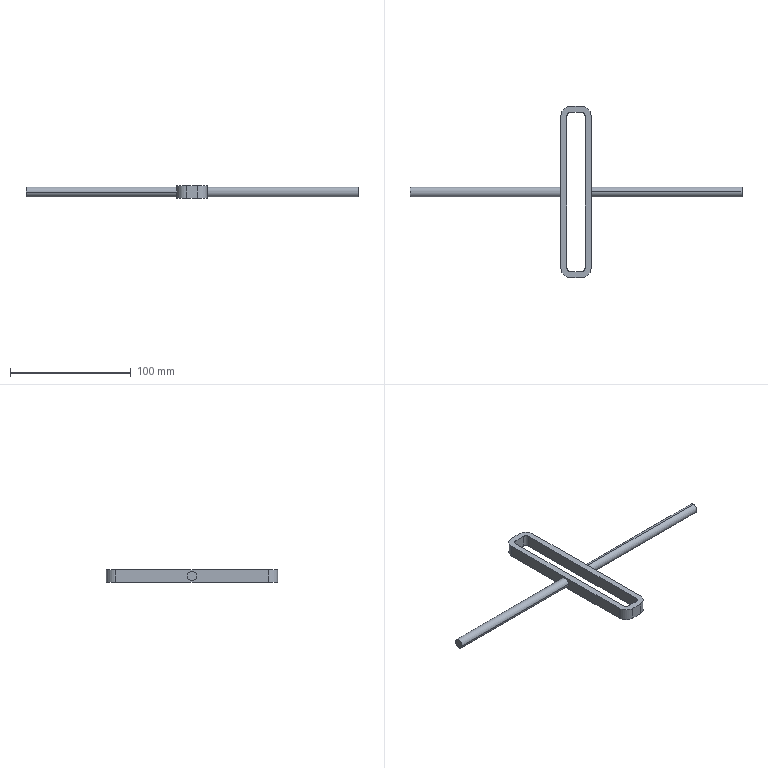Part | SolidWorks | features ICE 2, Extrusion 1 | 1 solid | 24 faces | box 275 x 142 x 10 mm | volume 27794 mm3 | cylinder 12 | plane 12 | commonest cylinder face diameters 6 x4 8 x4 16 x4
STEP:
#1=CARTESIAN_POINT('',(-137.5,-4.,5.));
#2=VERTEX_POINT('',#1);
#3=CARTESIAN_POINT('',(-137.5,4.,5.));
#4=VERTEX_POINT('',#3);
#5=CARTESIAN_POINT('',(-137.5,0.,5.));
#6=DIRECTION('',(-1.,0.,0.));
#7=DIRECTION('',(0.,-1.,0.));
#8=AXIS2_PLACEMENT_3D('',#5,#6,#7);
#9=CIRCLE('',#8,4.);
#10=EDGE_CURVE('',#2,#4,#9,.T.);
#11=ORIENTED_EDGE('',*,*,#10,.F.);
#12=CARTESIAN_POINT('',(-12.5,-4.,5.));
#13=VERTEX_POINT('',#12);
#14=CARTESIAN_POINT('',(-137.5,-4.,5.));
#15=DIRECTION('',(1.,0.,0.));
#16=VECTOR('',#15,1000.);
#17=LINE('',#14,#16);
#18=EDGE_CURVE('',#2,#13,#17,.T.);
#19=ORIENTED_EDGE('',*,*,#18,.T.);
#20=CARTESIAN_POINT('',(-12.5,4.,5.));
#21=VERTEX_POINT('',#20);
#22=CARTESIAN_POINT('',(-12.5,0.,5.));
#23=DIRECTION('',(-1.,0.,0.));
#24=DIRECTION('',(0.,1.,0.));
#25=AXIS2_PLACEMENT_3D('',#22,#23,#24);
#26=CIRCLE('',#25,4.);
#27=EDGE_CURVE('',#13,#21,#26,.T.);
#28=ORIENTED_EDGE('',*,*,#27,.T.);
#29=CARTESIAN_POINT('',(-137.5,4.,5.));
#30=DIRECTION('',(1.,0.,0.));
#31=VECTOR('',#30,1000.);
#32=LINE('',#29,#31);
#33=EDGE_CURVE('',#4,#21,#32,.T.);
#34=ORIENTED_EDGE('',*,*,#33,.F.);
#35=EDGE_LOOP('',(#11,#19,#28,#34));
#36=FACE_OUTER_BOUND('',#35,.T.);
#37=CARTESIAN_POINT('',(-137.5,0.,5.));
#38=DIRECTION('',(1.,0.,0.));
#39=DIRECTION('',(0.,1.,0.));
#40=AXIS2_PLACEMENT_3D('',#37,#38,#39);
#41=CYLINDRICAL_SURFACE('',#40,4.);
#42=ADVANCED_FACE('',(#36),#41,.T.);
#43=CARTESIAN_POINT('',(137.5,0.,1.));
#44=VERTEX_POINT('',#43);
#45=CARTESIAN_POINT('',(137.5,0.,9.));
#46=VERTEX_POINT('',#45);
#47=CARTESIAN_POINT('',(137.5,0.,5.));
#48=DIRECTION('',(1.,0.,0.));
#49=DIRECTION('',(0.,0.,-1.));
#50=AXIS2_PLACEMENT_3D('',#47,#48,#49);
#51=CIRCLE('',#50,4.);
#52=EDGE_CURVE('',#44,#46,#51,.T.);
#53=ORIENTED_EDGE('',*,*,#52,.F.);
#54=CARTESIAN_POINT('',(12.5,0.,1.));
#55=VERTEX_POINT('',#54);
#56=CARTESIAN_POINT('',(137.5,0.,1.));
#57=DIRECTION('',(-1.,0.,0.));
#58=VECTOR('',#57,1000.);
#59=LINE('',#56,#58);
#60=EDGE_CURVE('',#44,#55,#59,.T.);
#61=ORIENTED_EDGE('',*,*,#60,.T.);
#62=CARTESIAN_POINT('',(12.5,0.,9.));
#63=VERTEX_POINT('',#62);
#64=CARTESIAN_POINT('',(12.5,0.,5.));
#65=DIRECTION('',(1.,0.,0.));
#66=DIRECTION('',(0.,-1.,0.));
#67=AXIS2_PLACEMENT_3D('',#64,#65,#66);
#68=CIRCLE('',#67,4.);
#69=EDGE_CURVE('',#55,#63,#68,.T.);
#70=ORIENTED_EDGE('',*,*,#69,.T.);
#71=CARTESIAN_POINT('',(137.5,0.,9.));
#72=DIRECTION('',(-1.,0.,0.));
#73=VECTOR('',#72,1000.);
#74=LINE('',#71,#73);
#75=EDGE_CURVE('',#46,#63,#74,.T.);
#76=ORIENTED_EDGE('',*,*,#75,.F.);
#77=EDGE_LOOP('',(#53,#61,#70,#76));
#78=FACE_OUTER_BOUND('',#77,.T.);
#79=CARTESIAN_POINT('',(137.5,0.,5.));
#80=DIRECTION('',(-1.,0.,0.));
#81=DIRECTION('',(0.,0.,1.));
#82=AXIS2_PLACEMENT_3D('',#79,#80,#81);
#83=CYLINDRICAL_SURFACE('',#82,4.);
#84=ADVANCED_FACE('',(#78),#83,.T.);
#85=CARTESIAN_POINT('',(-4.5,71.,10.));
#86=VERTEX_POINT('',#85);
#87=CARTESIAN_POINT('',(-12.5,63.,10.));
#88=VERTEX_POINT('',#87);
#89=CARTESIAN_POINT('',(-4.5,63.,10.));
#90=DIRECTION('',(0.,0.,1.));
#91=DIRECTION('',(1.,0.,0.));
#92=AXIS2_PLACEMENT_3D('',#89,#90,#91);
#93=CIRCLE('',#92,8.);
#94=EDGE_CURVE('',#86,#88,#93,.T.);
#95=ORIENTED_EDGE('',*,*,#94,.T.);
#96=CARTESIAN_POINT('',(-12.5,-63.,10.));
#97=VERTEX_POINT('',#96);
#98=CARTESIAN_POINT('',(-12.5,63.,10.));
#99=DIRECTION('',(0.,-1.,0.));
#100=VECTOR('',#99,1000.);
#101=LINE('',#98,#100);
#102=EDGE_CURVE('',#88,#97,#101,.T.);
#103=ORIENTED_EDGE('',*,*,#102,.T.);
#104=CARTESIAN_POINT('',(-4.5,-71.,10.));
#105=VERTEX_POINT('',#104);
#106=CARTESIAN_POINT('',(-4.5,-63.,10.));
#107=DIRECTION('',(0.,0.,1.));
#108=DIRECTION('',(1.,0.,0.));
#109=AXIS2_PLACEMENT_3D('',#106,#107,#108);
#110=CIRCLE('',#109,8.);
#111=EDGE_CURVE('',#97,#105,#110,.T.);
#112=ORIENTED_EDGE('',*,*,#111,.T.);
#113=CARTESIAN_POINT('',(4.5,-71.,10.));
#114=VERTEX_POINT('',#113);
#115=CARTESIAN_POINT('',(-4.5,-71.,10.));
#116=DIRECTION('',(1.,0.,0.));
#117=VECTOR('',#116,1000.);
#118=LINE('',#115,#117);
#119=EDGE_CURVE('',#105,#114,#118,.T.);
#120=ORIENTED_EDGE('',*,*,#119,.T.);
#121=CARTESIAN_POINT('',(12.5,-63.,10.));
#122=VERTEX_POINT('',#121);
#123=CARTESIAN_POINT('',(4.5,-63.,10.));
#124=DIRECTION('',(0.,0.,1.));
#125=DIRECTION('',(1.,0.,0.));
#126=AXIS2_PLACEMENT_3D('',#123,#124,#125);
#127=CIRCLE('',#126,8.);
#128=EDGE_CURVE('',#114,#122,#127,.T.);
#129=ORIENTED_EDGE('',*,*,#128,.T.);
#130=CARTESIAN_POINT('',(12.5,63.,10.));
#131=VERTEX_POINT('',#130);
#132=CARTESIAN_POINT('',(12.5,63.,10.));
#133=DIRECTION('',(0.,1.,0.));
#134=VECTOR('',#133,1000.);
#135=LINE('',#132,#134);
#136=EDGE_CURVE('',#122,#131,#135,.T.);
#137=ORIENTED_EDGE('',*,*,#136,.T.);
#138=CARTESIAN_POINT('',(4.5,71.,10.));
#139=VERTEX_POINT('',#138);
#140=CARTESIAN_POINT('',(4.5,63.,10.));
#141=DIRECTION('',(0.,0.,1.));
#142=DIRECTION('',(-1.,0.,0.));
#143=AXIS2_PLACEMENT_3D('',#140,#141,#142);
#144=CIRCLE('',#143,8.);
#145=EDGE_CURVE('',#131,#139,#144,.T.);
#146=ORIENTED_EDGE('',*,*,#145,.T.);
#147=CARTESIAN_POINT('',(-4.5,71.,10.));
#148=DIRECTION('',(-1.,0.,0.));
#149=VECTOR('',#148,1000.);
#150=LINE('',#147,#149);
#151=EDGE_CURVE('',#139,#86,#150,.T.);
#152=ORIENTED_EDGE('',*,*,#151,.T.);
#153=EDGE_LOOP('',(#95,#103,#112,#120,#129,#137,#146,#152));
#154=FACE_OUTER_BOUND('',#153,.T.);
#155=CARTESIAN_POINT('',(-4.5,-66.,10.));
#156=VERTEX_POINT('',#155);
#157=CARTESIAN_POINT('',(4.5,-66.,10.));
#158=VERTEX_POINT('',#157);
#159=CARTESIAN_POINT('',(-4.5,-66.,10.));
#160=DIRECTION('',(1.,0.,0.));
#161=VECTOR('',#160,1000.);
#162=LINE('',#159,#161);
#163=EDGE_CURVE('',#156,#158,#162,.T.);
#164=ORIENTED_EDGE('',*,*,#163,.F.);
#165=CARTESIAN_POINT('',(-7.5,-63.,10.));
#166=VERTEX_POINT('',#165);
#167=CARTESIAN_POINT('',(-4.5,-63.,10.));
#168=DIRECTION('',(0.,0.,1.));
#169=DIRECTION('',(1.,0.,0.));
#170=AXIS2_PLACEMENT_3D('',#167,#168,#169);
#171=CIRCLE('',#170,3.);
#172=EDGE_CURVE('',#166,#156,#171,.T.);
#173=ORIENTED_EDGE('',*,*,#172,.F.);
#174=CARTESIAN_POINT('',(-7.5,63.,10.));
#175=VERTEX_POINT('',#174);
#176=CARTESIAN_POINT('',(-7.5,63.,10.));
#177=DIRECTION('',(0.,-1.,0.));
#178=VECTOR('',#177,1000.);
#179=LINE('',#176,#178);
#180=EDGE_CURVE('',#175,#166,#179,.T.);
#181=ORIENTED_EDGE('',*,*,#180,.F.);
#182=CARTESIAN_POINT('',(-4.5,66.,10.));
#183=VERTEX_POINT('',#182);
#184=CARTESIAN_POINT('',(-4.5,63.,10.));
#185=DIRECTION('',(0.,0.,1.));
#186=DIRECTION('',(1.,0.,0.));
#187=AXIS2_PLACEMENT_3D('',#184,#185,#186);
#188=CIRCLE('',#187,3.);
#189=EDGE_CURVE('',#183,#175,#188,.T.);
#190=ORIENTED_EDGE('',*,*,#189,.F.);
#191=CARTESIAN_POINT('',(4.5,66.,10.));
#192=VERTEX_POINT('',#191);
#193=CARTESIAN_POINT('',(-4.5,66.,10.));
#194=DIRECTION('',(-1.,0.,0.));
#195=VECTOR('',#194,1000.);
#196=LINE('',#193,#195);
#197=EDGE_CURVE('',#192,#183,#196,.T.);
#198=ORIENTED_EDGE('',*,*,#197,.F.);
#199=CARTESIAN_POINT('',(7.5,63.,10.));
#200=VERTEX_POINT('',#199);
#201=CARTESIAN_POINT('',(4.5,63.,10.));
#202=DIRECTION('',(0.,0.,1.));
#203=DIRECTION('',(-1.,0.,0.));
#204=AXIS2_PLACEMENT_3D('',#201,#202,#203);
#205=CIRCLE('',#204,3.);
#206=EDGE_CURVE('',#200,#192,#205,.T.);
#207=ORIENTED_EDGE('',*,*,#206,.F.);
#208=CARTESIAN_POINT('',(7.5,-63.,10.));
#209=VERTEX_POINT('',#208);
#210=CARTESIAN_POINT('',(7.5,63.,10.));
#211=DIRECTION('',(0.,1.,0.));
#212=VECTOR('',#211,1000.);
#213=LINE('',#210,#212);
#214=EDGE_CURVE('',#209,#200,#213,.T.);
#215=ORIENTED_EDGE('',*,*,#214,.F.);
#216=CARTESIAN_POINT('',(4.5,-63.,10.));
#217=DIRECTION('',(0.,0.,1.));
#218=DIRECTION('',(1.,0.,0.));
#219=AXIS2_PLACEMENT_3D('',#216,#217,#218);
#220=CIRCLE('',#219,3.);
#221=EDGE_CURVE('',#158,#209,#220,.T.);
#222=ORIENTED_EDGE('',*,*,#221,.F.);
#223=EDGE_LOOP('',(#164,#173,#181,#190,#198,#207,#215,#222));
#224=FACE_BOUND('',#223,.T.);
#225=CARTESIAN_POINT('',(-4.5,63.,10.));
#226=DIRECTION('',(0.,0.,1.));
#227=DIRECTION('',(1.,0.,0.));
#228=AXIS2_PLACEMENT_3D('',#225,#226,#227);
#229=PLANE('',#228);
#230=ADVANCED_FACE('',(#154,#224),#229,.T.);
#231=CARTESIAN_POINT('',(-4.5,71.,0.));
#232=VERTEX_POINT('',#231);
#233=CARTESIAN_POINT('',(-12.5,63.,0.));
#234=VERTEX_POINT('',#233);
#235=CARTESIAN_POINT('',(-4.5,63.,0.));
#236=DIRECTION('',(0.,0.,1.));
#237=DIRECTION('',(1.,0.,0.));
#238=AXIS2_PLACEMENT_3D('',#235,#236,#237);
#239=CIRCLE('',#238,8.);
#240=EDGE_CURVE('',#232,#234,#239,.T.);
#241=ORIENTED_EDGE('',*,*,#240,.F.);
#242=CARTESIAN_POINT('',(4.5,71.,0.));
#243=VERTEX_POINT('',#242);
#244=CARTESIAN_POINT('',(-4.5,71.,0.));
#245=DIRECTION('',(-1.,0.,0.));
#246=VECTOR('',#245,1000.);
#247=LINE('',#244,#246);
#248=EDGE_CURVE('',#243,#232,#247,.T.);
#249=ORIENTED_EDGE('',*,*,#248,.F.);
#250=CARTESIAN_POINT('',(12.5,63.,0.));
#251=VERTEX_POINT('',#250);
#252=CARTESIAN_POINT('',(4.5,63.,0.));
#253=DIRECTION('',(0.,0.,1.));
#254=DIRECTION('',(-1.,0.,0.));
#255=AXIS2_PLACEMENT_3D('',#252,#253,#254);
#256=CIRCLE('',#255,8.);
#257=EDGE_CURVE('',#251,#243,#256,.T.);
#258=ORIENTED_EDGE('',*,*,#257,.F.);
#259=CARTESIAN_POINT('',(12.5,-63.,0.));
#260=VERTEX_POINT('',#259);
#261=CARTESIAN_POINT('',(12.5,63.,0.));
#262=DIRECTION('',(0.,1.,0.));
#263=VECTOR('',#262,1000.);
#264=LINE('',#261,#263);
#265=EDGE_CURVE('',#260,#251,#264,.T.);
#266=ORIENTED_EDGE('',*,*,#265,.F.);
#267=CARTESIAN_POINT('',(4.5,-71.,0.));
#268=VERTEX_POINT('',#267);
#269=CARTESIAN_POINT('',(4.5,-63.,0.));
#270=DIRECTION('',(0.,0.,1.));
#271=DIRECTION('',(1.,0.,0.));
#272=AXIS2_PLACEMENT_3D('',#269,#270,#271);
#273=CIRCLE('',#272,8.);
#274=EDGE_CURVE('',#268,#260,#273,.T.);
#275=ORIENTED_EDGE('',*,*,#274,.F.);
#276=CARTESIAN_POINT('',(-4.5,-71.,0.));
#277=VERTEX_POINT('',#276);
#278=CARTESIAN_POINT('',(-4.5,-71.,0.));
#279=DIRECTION('',(1.,0.,0.));
#280=VECTOR('',#279,1000.);
#281=LINE('',#278,#280);
#282=EDGE_CURVE('',#277,#268,#281,.T.);
#283=ORIENTED_EDGE('',*,*,#282,.F.);
#284=CARTESIAN_POINT('',(-12.5,-63.,0.));
#285=VERTEX_POINT('',#284);
#286=CARTESIAN_POINT('',(-4.5,-63.,0.));
#287=DIRECTION('',(0.,0.,1.));
#288=DIRECTION('',(1.,0.,0.));
#289=AXIS2_PLACEMENT_3D('',#286,#287,#288);
#290=CIRCLE('',#289,8.);
#291=EDGE_CURVE('',#285,#277,#290,.T.);
#292=ORIENTED_EDGE('',*,*,#291,.F.);
#293=CARTESIAN_POINT('',(-12.5,63.,0.));
#294=DIRECTION('',(0.,-1.,0.));
#295=VECTOR('',#294,1000.);
#296=LINE('',#293,#295);
#297=EDGE_CURVE('',#234,#285,#296,.T.);
#298=ORIENTED_EDGE('',*,*,#297,.F.);
#299=EDGE_LOOP('',(#241,#249,#258,#266,#275,#283,#292,#298));
#300=FACE_OUTER_BOUND('',#299,.T.);
#301=CARTESIAN_POINT('',(-7.5,-63.,0.));
#302=VERTEX_POINT('',#301);
#303=CARTESIAN_POINT('',(-4.5,-66.,0.));
#304=VERTEX_POINT('',#303);
#305=CARTESIAN_POINT('',(-4.5,-63.,0.));
#306=DIRECTION('',(0.,0.,1.));
#307=DIRECTION('',(1.,0.,0.));
#308=AXIS2_PLACEMENT_3D('',#305,#306,#307);
#309=CIRCLE('',#308,3.);
#310=EDGE_CURVE('',#302,#304,#309,.T.);
#311=ORIENTED_EDGE('',*,*,#310,.T.);
#312=CARTESIAN_POINT('',(4.5,-66.,0.));
#313=VERTEX_POINT('',#312);
#314=CARTESIAN_POINT('',(-4.5,-66.,0.));
#315=DIRECTION('',(1.,0.,0.));
#316=VECTOR('',#315,1000.);
#317=LINE('',#314,#316);
#318=EDGE_CURVE('',#304,#313,#317,.T.);
#319=ORIENTED_EDGE('',*,*,#318,.T.);
#320=CARTESIAN_POINT('',(7.5,-63.,0.));
#321=VERTEX_POINT('',#320);
#322=CARTESIAN_POINT('',(4.5,-63.,0.));
#323=DIRECTION('',(0.,0.,1.));
#324=DIRECTION('',(1.,0.,0.));
#325=AXIS2_PLACEMENT_3D('',#322,#323,#324);
#326=CIRCLE('',#325,3.);
#327=EDGE_CURVE('',#313,#321,#326,.T.);
#328=ORIENTED_EDGE('',*,*,#327,.T.);
#329=CARTESIAN_POINT('',(7.5,63.,0.));
#330=VERTEX_POINT('',#329);
#331=CARTESIAN_POINT('',(7.5,63.,0.));
#332=DIRECTION('',(0.,1.,0.));
#333=VECTOR('',#332,1000.);
#334=LINE('',#331,#333);
#335=EDGE_CURVE('',#321,#330,#334,.T.);
#336=ORIENTED_EDGE('',*,*,#335,.T.);
#337=CARTESIAN_POINT('',(4.5,66.,0.));
#338=VERTEX_POINT('',#337);
#339=CARTESIAN_POINT('',(4.5,63.,0.));
#340=DIRECTION('',(0.,0.,1.));
#341=DIRECTION('',(-1.,0.,0.));
#342=AXIS2_PLACEMENT_3D('',#339,#340,#341);
#343=CIRCLE('',#342,3.);
#344=EDGE_CURVE('',#330,#338,#343,.T.);
#345=ORIENTED_EDGE('',*,*,#344,.T.);
#346=CARTESIAN_POINT('',(-4.5,66.,0.));
#347=VERTEX_POINT('',#346);
#348=CARTESIAN_POINT('',(-4.5,66.,0.));
#349=DIRECTION('',(-1.,0.,0.));
#350=VECTOR('',#349,1000.);
#351=LINE('',#348,#350);
#352=EDGE_CURVE('',#338,#347,#351,.T.);
#353=ORIENTED_EDGE('',*,*,#352,.T.);
#354=CARTESIAN_POINT('',(-7.5,63.,0.));
#355=VERTEX_POINT('',#354);
#356=CARTESIAN_POINT('',(-4.5,63.,0.));
#357=DIRECTION('',(0.,0.,1.));
#358=DIRECTION('',(1.,0.,0.));
#359=AXIS2_PLACEMENT_3D('',#356,#357,#358);
#360=CIRCLE('',#359,3.);
#361=EDGE_CURVE('',#347,#355,#360,.T.);
#362=ORIENTED_EDGE('',*,*,#361,.T.);
#363=CARTESIAN_POINT('',(-7.5,63.,0.));
#364=DIRECTION('',(0.,-1.,0.));
#365=VECTOR('',#364,1000.);
#366=LINE('',#363,#365);
#367=EDGE_CURVE('',#355,#302,#366,.T.);
#368=ORIENTED_EDGE('',*,*,#367,.T.);
#369=EDGE_LOOP('',(#311,#319,#328,#336,#345,#353,#362,#368));
#370=FACE_BOUND('',#369,.T.);
#371=CARTESIAN_POINT('',(-4.5,63.,0.));
#372=DIRECTION('',(0.,0.,1.));
#373=DIRECTION('',(1.,0.,0.));
#374=AXIS2_PLACEMENT_3D('',#371,#372,#373);
#375=PLANE('',#374);
#376=ADVANCED_FACE('',(#300,#370),#375,.F.);
#377=ORIENTED_EDGE('',*,*,#240,.T.);
#378=CARTESIAN_POINT('',(-12.5,63.,10.));
#379=DIRECTION('',(0.,0.,-1.));
#380=VECTOR('',#379,1000.);
#381=LINE('',#378,#380);
#382=EDGE_CURVE('',#88,#234,#381,.T.);
#383=ORIENTED_EDGE('',*,*,#382,.F.);
#384=ORIENTED_EDGE('',*,*,#94,.F.);
#385=CARTESIAN_POINT('',(-4.5,71.,10.));
#386=DIRECTION('',(0.,0.,-1.));
#387=VECTOR('',#386,1000.);
#388=LINE('',#385,#387);
#389=EDGE_CURVE('',#86,#232,#388,.T.);
#390=ORIENTED_EDGE('',*,*,#389,.T.);
#391=EDGE_LOOP('',(#377,#383,#384,#390));
#392=FACE_OUTER_BOUND('',#391,.T.);
#393=CARTESIAN_POINT('',(-4.5,63.,10.));
#394=DIRECTION('',(0.,0.,-1.));
#395=DIRECTION('',(-1.,0.,0.));
#396=AXIS2_PLACEMENT_3D('',#393,#394,#395);
#397=CYLINDRICAL_SURFACE('',#396,8.);
#398=ADVANCED_FACE('',(#392),#397,.T.);
#399=CARTESIAN_POINT('',(-12.5,0.,5.));
#400=DIRECTION('',(-1.,0.,0.));
#401=DIRECTION('',(0.,1.,0.));
#402=AXIS2_PLACEMENT_3D('',#399,#400,#401);
#403=CIRCLE('',#402,4.);
#404=EDGE_CURVE('',#21,#13,#403,.T.);
#405=ORIENTED_EDGE('',*,*,#404,.F.);
#406=ORIENTED_EDGE('',*,*,#27,.F.);
#407=EDGE_LOOP('',(#405,#406));
#408=FACE_BOUND('',#407,.T.);
#409=ORIENTED_EDGE('',*,*,#297,.T.);
#410=CARTESIAN_POINT('',(-12.5,-63.,10.));
#411=DIRECTION('',(0.,0.,-1.));
#412=VECTOR('',#411,1000.);
#413=LINE('',#410,#412);
#414=EDGE_CURVE('',#97,#285,#413,.T.);
#415=ORIENTED_EDGE('',*,*,#414,.F.);
#416=ORIENTED_EDGE('',*,*,#102,.F.);
#417=ORIENTED_EDGE('',*,*,#382,.T.);
#418=EDGE_LOOP('',(#409,#415,#416,#417));
#419=FACE_OUTER_BOUND('',#418,.T.);
#420=CARTESIAN_POINT('',(-12.5,63.,10.));
#421=DIRECTION('',(1.,0.,0.));
#422=DIRECTION('',(0.,1.,0.));
#423=AXIS2_PLACEMENT_3D('',#420,#421,#422);
#424=PLANE('',#423);
#425=ADVANCED_FACE('',(#408,#419),#424,.F.);
#426=ORIENTED_EDGE('',*,*,#291,.T.);
#427=CARTESIAN_POINT('',(-4.5,-71.,10.));
#428=DIRECTION('',(0.,0.,-1.));
#429=VECTOR('',#428,1000.);
#430=LINE('',#427,#429);
#431=EDGE_CURVE('',#105,#277,#430,.T.);
#432=ORIENTED_EDGE('',*,*,#431,.F.);
#433=ORIENTED_EDGE('',*,*,#111,.F.);
#434=ORIENTED_EDGE('',*,*,#414,.T.);
#435=EDGE_LOOP('',(#426,#432,#433,#434));
#436=FACE_OUTER_BOUND('',#435,.T.);
#437=CARTESIAN_POINT('',(-4.5,-63.,10.));
#438=DIRECTION('',(0.,0.,-1.));
#439=DIRECTION('',(-1.,0.,0.));
#440=AXIS2_PLACEMENT_3D('',#437,#438,#439);
#441=CYLINDRICAL_SURFACE('',#440,8.);
#442=ADVANCED_FACE('',(#436),#441,.T.);
#443=ORIENTED_EDGE('',*,*,#282,.T.);
#444=CARTESIAN_POINT('',(4.5,-71.,10.));
#445=DIRECTION('',(0.,0.,-1.));
#446=VECTOR('',#445,1000.);
#447=LINE('',#444,#446);
#448=EDGE_CURVE('',#114,#268,#447,.T.);
#449=ORIENTED_EDGE('',*,*,#448,.F.);
#450=ORIENTED_EDGE('',*,*,#119,.F.);
#451=ORIENTED_EDGE('',*,*,#431,.T.);
#452=EDGE_LOOP('',(#443,#449,#450,#451));
#453=FACE_OUTER_BOUND('',#452,.T.);
#454=CARTESIAN_POINT('',(-4.5,-71.,10.));
#455=DIRECTION('',(0.,1.,0.));
#456=DIRECTION('',(0.,0.,1.));
#457=AXIS2_PLACEMENT_3D('',#454,#455,#456);
#458=PLANE('',#457);
#459=ADVANCED_FACE('',(#453),#458,.F.);
#460=ORIENTED_EDGE('',*,*,#274,.T.);
#461=CARTESIAN_POINT('',(12.5,-63.,10.));
#462=DIRECTION('',(0.,0.,-1.));
#463=VECTOR('',#462,1000.);
#464=LINE('',#461,#463);
#465=EDGE_CURVE('',#122,#260,#464,.T.);
#466=ORIENTED_EDGE('',*,*,#465,.F.);
#467=ORIENTED_EDGE('',*,*,#128,.F.);
#468=ORIENTED_EDGE('',*,*,#448,.T.);
#469=EDGE_LOOP('',(#460,#466,#467,#468));
#470=FACE_OUTER_BOUND('',#469,.T.);
#471=CARTESIAN_POINT('',(4.5,-63.,10.));
#472=DIRECTION('',(0.,0.,-1.));
#473=DIRECTION('',(-1.,0.,0.));
#474=AXIS2_PLACEMENT_3D('',#471,#472,#473);
#475=CYLINDRICAL_SURFACE('',#474,8.);
#476=ADVANCED_FACE('',(#470),#475,.T.);
#477=CARTESIAN_POINT('',(12.5,0.,5.));
#478=DIRECTION('',(1.,0.,0.));
#479=DIRECTION('',(0.,-1.,0.));
#480=AXIS2_PLACEMENT_3D('',#477,#478,#479);
#481=CIRCLE('',#480,4.);
#482=EDGE_CURVE('',#63,#55,#481,.T.);
#483=ORIENTED_EDGE('',*,*,#482,.F.);
#484=ORIENTED_EDGE('',*,*,#69,.F.);
#485=EDGE_LOOP('',(#483,#484));
#486=FACE_BOUND('',#485,.T.);
#487=ORIENTED_EDGE('',*,*,#265,.T.);
#488=CARTESIAN_POINT('',(12.5,63.,10.));
#489=DIRECTION('',(0.,0.,-1.));
#490=VECTOR('',#489,1000.);
#491=LINE('',#488,#490);
#492=EDGE_CURVE('',#131,#251,#491,.T.);
#493=ORIENTED_EDGE('',*,*,#492,.F.);
#494=ORIENTED_EDGE('',*,*,#136,.F.);
#495=ORIENTED_EDGE('',*,*,#465,.T.);
#496=EDGE_LOOP('',(#487,#493,#494,#495));
#497=FACE_OUTER_BOUND('',#496,.T.);
#498=CARTESIAN_POINT('',(12.5,63.,10.));
#499=DIRECTION('',(-1.,0.,0.));
#500=DIRECTION('',(0.,-1.,0.));
#501=AXIS2_PLACEMENT_3D('',#498,#499,#500);
#502=PLANE('',#501);
#503=ADVANCED_FACE('',(#486,#497),#502,.F.);
#504=ORIENTED_EDGE('',*,*,#257,.T.);
#505=CARTESIAN_POINT('',(4.5,71.,10.));
#506=DIRECTION('',(0.,0.,-1.));
#507=VECTOR('',#506,1000.);
#508=LINE('',#505,#507);
#509=EDGE_CURVE('',#139,#243,#508,.T.);
#510=ORIENTED_EDGE('',*,*,#509,.F.);
#511=ORIENTED_EDGE('',*,*,#145,.F.);
#512=ORIENTED_EDGE('',*,*,#492,.T.);
#513=EDGE_LOOP('',(#504,#510,#511,#512));
#514=FACE_OUTER_BOUND('',#513,.T.);
#515=CARTESIAN_POINT('',(4.5,63.,10.));
#516=DIRECTION('',(0.,0.,-1.));
#517=DIRECTION('',(-1.,0.,0.));
#518=AXIS2_PLACEMENT_3D('',#515,#516,#517);
#519=CYLINDRICAL_SURFACE('',#518,8.);
#520=ADVANCED_FACE('',(#514),#519,.T.);
#521=ORIENTED_EDGE('',*,*,#248,.T.);
#522=ORIENTED_EDGE('',*,*,#389,.F.);
#523=ORIENTED_EDGE('',*,*,#151,.F.);
#524=ORIENTED_EDGE('',*,*,#509,.T.);
#525=EDGE_LOOP('',(#521,#522,#523,#524));
#526=FACE_OUTER_BOUND('',#525,.T.);
#527=CARTESIAN_POINT('',(-4.5,71.,10.));
#528=DIRECTION('',(0.,-1.,0.));
#529=DIRECTION('',(0.,0.,-1.));
#530=AXIS2_PLACEMENT_3D('',#527,#528,#529);
#531=PLANE('',#530);
#532=ADVANCED_FACE('',(#526),#531,.F.);
#533=ORIENTED_EDGE('',*,*,#310,.F.);
#534=CARTESIAN_POINT('',(-7.5,-63.,10.));
#535=DIRECTION('',(0.,0.,-1.));
#536=VECTOR('',#535,1000.);
#537=LINE('',#534,#536);
#538=EDGE_CURVE('',#166,#302,#537,.T.);
#539=ORIENTED_EDGE('',*,*,#538,.F.);
#540=ORIENTED_EDGE('',*,*,#172,.T.);
#541=CARTESIAN_POINT('',(-4.5,-66.,10.));
#542=DIRECTION('',(0.,0.,-1.));
#543=VECTOR('',#542,1000.);
#544=LINE('',#541,#543);
#545=EDGE_CURVE('',#156,#304,#544,.T.);
#546=ORIENTED_EDGE('',*,*,#545,.T.);
#547=EDGE_LOOP('',(#533,#539,#540,#546));
#548=FACE_OUTER_BOUND('',#547,.T.);
#549=CARTESIAN_POINT('',(-4.5,-63.,10.));
#550=DIRECTION('',(0.,0.,-1.));
#551=DIRECTION('',(-1.,0.,0.));
#552=AXIS2_PLACEMENT_3D('',#549,#550,#551);
#553=CYLINDRICAL_SURFACE('',#552,3.);
#554=ADVANCED_FACE('',(#548),#553,.F.);
#555=ORIENTED_EDGE('',*,*,#318,.F.);
#556=ORIENTED_EDGE('',*,*,#545,.F.);
#557=ORIENTED_EDGE('',*,*,#163,.T.);
#558=CARTESIAN_POINT('',(4.5,-66.,10.));
#559=DIRECTION('',(0.,0.,-1.));
#560=VECTOR('',#559,1000.);
#561=LINE('',#558,#560);
#562=EDGE_CURVE('',#158,#313,#561,.T.);
#563=ORIENTED_EDGE('',*,*,#562,.T.);
#564=EDGE_LOOP('',(#555,#556,#557,#563));
#565=FACE_OUTER_BOUND('',#564,.T.);
#566=CARTESIAN_POINT('',(-4.5,-66.,10.));
#567=DIRECTION('',(0.,1.,0.));
#568=DIRECTION('',(0.,0.,1.));
#569=AXIS2_PLACEMENT_3D('',#566,#567,#568);
#570=PLANE('',#569);
#571=ADVANCED_FACE('',(#565),#570,.T.);
#572=ORIENTED_EDGE('',*,*,#327,.F.);
#573=ORIENTED_EDGE('',*,*,#562,.F.);
#574=ORIENTED_EDGE('',*,*,#221,.T.);
#575=CARTESIAN_POINT('',(7.5,-63.,10.));
#576=DIRECTION('',(0.,0.,-1.));
#577=VECTOR('',#576,1000.);
#578=LINE('',#575,#577);
#579=EDGE_CURVE('',#209,#321,#578,.T.);
#580=ORIENTED_EDGE('',*,*,#579,.T.);
#581=EDGE_LOOP('',(#572,#573,#574,#580));
#582=FACE_OUTER_BOUND('',#581,.T.);
#583=CARTESIAN_POINT('',(4.5,-63.,10.));
#584=DIRECTION('',(0.,0.,-1.));
#585=DIRECTION('',(-1.,0.,0.));
#586=AXIS2_PLACEMENT_3D('',#583,#584,#585);
#587=CYLINDRICAL_SURFACE('',#586,3.);
#588=ADVANCED_FACE('',(#582),#587,.F.);
#589=ORIENTED_EDGE('',*,*,#335,.F.);
#590=ORIENTED_EDGE('',*,*,#579,.F.);
#591=ORIENTED_EDGE('',*,*,#214,.T.);
#592=CARTESIAN_POINT('',(7.5,63.,10.));
#593=DIRECTION('',(0.,0.,-1.));
#594=VECTOR('',#593,1000.);
#595=LINE('',#592,#594);
#596=EDGE_CURVE('',#200,#330,#595,.T.);
#597=ORIENTED_EDGE('',*,*,#596,.T.);
#598=EDGE_LOOP('',(#589,#590,#591,#597));
#599=FACE_OUTER_BOUND('',#598,.T.);
#600=CARTESIAN_POINT('',(7.5,63.,10.));
#601=DIRECTION('',(-1.,0.,0.));
#602=DIRECTION('',(0.,-1.,0.));
#603=AXIS2_PLACEMENT_3D('',#600,#601,#602);
#604=PLANE('',#603);
#605=ADVANCED_FACE('',(#599),#604,.T.);
#606=ORIENTED_EDGE('',*,*,#344,.F.);
#607=ORIENTED_EDGE('',*,*,#596,.F.);
#608=ORIENTED_EDGE('',*,*,#206,.T.);
#609=CARTESIAN_POINT('',(4.5,66.,10.));
#610=DIRECTION('',(0.,0.,-1.));
#611=VECTOR('',#610,1000.);
#612=LINE('',#609,#611);
#613=EDGE_CURVE('',#192,#338,#612,.T.);
#614=ORIENTED_EDGE('',*,*,#613,.T.);
#615=EDGE_LOOP('',(#606,#607,#608,#614));
#616=FACE_OUTER_BOUND('',#615,.T.);
#617=CARTESIAN_POINT('',(4.5,63.,10.));
#618=DIRECTION('',(0.,0.,-1.));
#619=DIRECTION('',(-1.,0.,0.));
#620=AXIS2_PLACEMENT_3D('',#617,#618,#619);
#621=CYLINDRICAL_SURFACE('',#620,3.);
#622=ADVANCED_FACE('',(#616),#621,.F.);
#623=ORIENTED_EDGE('',*,*,#352,.F.);
#624=ORIENTED_EDGE('',*,*,#613,.F.);
#625=ORIENTED_EDGE('',*,*,#197,.T.);
#626=CARTESIAN_POINT('',(-4.5,66.,10.));
#627=DIRECTION('',(0.,0.,-1.));
#628=VECTOR('',#627,1000.);
#629=LINE('',#626,#628);
#630=EDGE_CURVE('',#183,#347,#629,.T.);
#631=ORIENTED_EDGE('',*,*,#630,.T.);
#632=EDGE_LOOP('',(#623,#624,#625,#631));
#633=FACE_OUTER_BOUND('',#632,.T.);
#634=CARTESIAN_POINT('',(-4.5,66.,10.));
#635=DIRECTION('',(0.,-1.,0.));
#636=DIRECTION('',(0.,0.,-1.));
#637=AXIS2_PLACEMENT_3D('',#634,#635,#636);
#638=PLANE('',#637);
#639=ADVANCED_FACE('',(#633),#638,.T.);
#640=ORIENTED_EDGE('',*,*,#361,.F.);
#641=ORIENTED_EDGE('',*,*,#630,.F.);
#642=ORIENTED_EDGE('',*,*,#189,.T.);
#643=CARTESIAN_POINT('',(-7.5,63.,10.));
#644=DIRECTION('',(0.,0.,-1.));
#645=VECTOR('',#644,1000.);
#646=LINE('',#643,#645);
#647=EDGE_CURVE('',#175,#355,#646,.T.);
#648=ORIENTED_EDGE('',*,*,#647,.T.);
#649=EDGE_LOOP('',(#640,#641,#642,#648));
#650=FACE_OUTER_BOUND('',#649,.T.);
#651=CARTESIAN_POINT('',(-4.5,63.,10.));
#652=DIRECTION('',(0.,0.,-1.));
#653=DIRECTION('',(-1.,0.,0.));
#654=AXIS2_PLACEMENT_3D('',#651,#652,#653);
#655=CYLINDRICAL_SURFACE('',#654,3.);
#656=ADVANCED_FACE('',(#650),#655,.F.);
#657=ORIENTED_EDGE('',*,*,#367,.F.);
#658=ORIENTED_EDGE('',*,*,#647,.F.);
#659=ORIENTED_EDGE('',*,*,#180,.T.);
#660=ORIENTED_EDGE('',*,*,#538,.T.);
#661=EDGE_LOOP('',(#657,#658,#659,#660));
#662=FACE_OUTER_BOUND('',#661,.T.);
#663=CARTESIAN_POINT('',(-7.5,63.,10.));
#664=DIRECTION('',(1.,0.,0.));
#665=DIRECTION('',(0.,1.,0.));
#666=AXIS2_PLACEMENT_3D('',#663,#664,#665);
#667=PLANE('',#666);
#668=ADVANCED_FACE('',(#662),#667,.T.);
#669=ORIENTED_EDGE('',*,*,#60,.F.);
#670=CARTESIAN_POINT('',(137.5,0.,5.));
#671=DIRECTION('',(1.,0.,0.));
#672=DIRECTION('',(0.,0.,-1.));
#673=AXIS2_PLACEMENT_3D('',#670,#671,#672);
#674=CIRCLE('',#673,4.);
#675=EDGE_CURVE('',#46,#44,#674,.T.);
#676=ORIENTED_EDGE('',*,*,#675,.F.);
#677=ORIENTED_EDGE('',*,*,#75,.T.);
#678=ORIENTED_EDGE('',*,*,#482,.T.);
#679=EDGE_LOOP('',(#669,#676,#677,#678));
#680=FACE_OUTER_BOUND('',#679,.T.);
#681=CARTESIAN_POINT('',(137.5,0.,5.));
#682=DIRECTION('',(-1.,0.,0.));
#683=DIRECTION('',(0.,0.,1.));
#684=AXIS2_PLACEMENT_3D('',#681,#682,#683);
#685=CYLINDRICAL_SURFACE('',#684,4.);
#686=ADVANCED_FACE('',(#680),#685,.T.);
#687=ORIENTED_EDGE('',*,*,#675,.T.);
#688=ORIENTED_EDGE('',*,*,#52,.T.);
#689=EDGE_LOOP('',(#687,#688));
#690=FACE_OUTER_BOUND('',#689,.T.);
#691=CARTESIAN_POINT('',(137.5,0.,5.));
#692=DIRECTION('',(1.,0.,0.));
#693=DIRECTION('',(0.,0.,-1.));
#694=AXIS2_PLACEMENT_3D('',#691,#692,#693);
#695=PLANE('',#694);
#696=ADVANCED_FACE('',(#690),#695,.T.);
#697=ORIENTED_EDGE('',*,*,#18,.F.);
#698=CARTESIAN_POINT('',(-137.5,0.,5.));
#699=DIRECTION('',(-1.,0.,0.));
#700=DIRECTION('',(0.,-1.,0.));
#701=AXIS2_PLACEMENT_3D('',#698,#699,#700);
#702=CIRCLE('',#701,4.);
#703=EDGE_CURVE('',#4,#2,#702,.T.);
#704=ORIENTED_EDGE('',*,*,#703,.F.);
#705=ORIENTED_EDGE('',*,*,#33,.T.);
#706=ORIENTED_EDGE('',*,*,#404,.T.);
#707=EDGE_LOOP('',(#697,#704,#705,#706));
#708=FACE_OUTER_BOUND('',#707,.T.);
#709=CARTESIAN_POINT('',(-137.5,0.,5.));
#710=DIRECTION('',(1.,0.,0.));
#711=DIRECTION('',(0.,1.,0.));
#712=AXIS2_PLACEMENT_3D('',#709,#710,#711);
#713=CYLINDRICAL_SURFACE('',#712,4.);
#714=ADVANCED_FACE('',(#708),#713,.T.);
#715=ORIENTED_EDGE('',*,*,#703,.T.);
#716=ORIENTED_EDGE('',*,*,#10,.T.);
#717=EDGE_LOOP('',(#715,#716));
#718=FACE_OUTER_BOUND('',#717,.T.);
#719=CARTESIAN_POINT('',(-137.5,0.,5.));
#720=DIRECTION('',(-1.,0.,0.));
#721=DIRECTION('',(0.,-1.,0.));
#722=AXIS2_PLACEMENT_3D('',#719,#720,#721);
#723=PLANE('',#722);
#724=ADVANCED_FACE('',(#718),#723,.T.);
#725=CLOSED_SHELL('',(#42,#84,#230,#376,#398,#425,#442,#459,#476,#503,#520,#532,#554,#571,#588,#605,#622,#639,#656,#668,#686,#696,#714,#724));
#726=MANIFOLD_SOLID_BREP('',#725);
#727=CARTESIAN_POINT('',(0.,0.,0.));
#728=DIRECTION('',(0.,0.,1.));
#729=DIRECTION('',(1.,0.,0.));
#730=AXIS2_PLACEMENT_3D('',#727,#728,#729);
#731=(LENGTH_UNIT()NAMED_UNIT(*)SI_UNIT(.MILLI.,.METRE.));
#732=UNCERTAINTY_MEASURE_WITH_UNIT(LENGTH_MEASURE(0.00001),#731,'','');
#733=(NAMED_UNIT(*)PLANE_ANGLE_UNIT()SI_UNIT($,.RADIAN.));
#734=(NAMED_UNIT(*)SI_UNIT($,.STERADIAN.)SOLID_ANGLE_UNIT());
#735=(GEOMETRIC_REPRESENTATION_CONTEXT(3)GLOBAL_UNCERTAINTY_ASSIGNED_CONTEXT((#732))GLOBAL_UNIT_ASSIGNED_CONTEXT((#731,#733,#734))REPRESENTATION_CONTEXT('',''));
#736=ADVANCED_BREP_SHAPE_REPRESENTATION('',(#726,#730),#735);